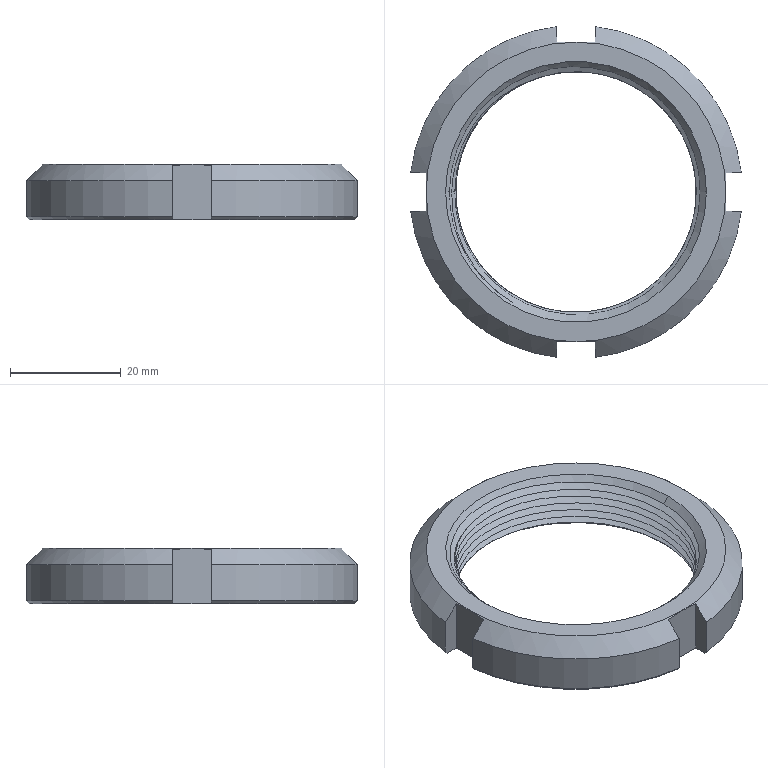Part | SolidWorks | features Chamfer 4, Helix 2, CirPattern 1, Extrusion 1, ICE 1, SweepCut 1 | 1 solid | 32 faces | box 59.59 x 59.59 x 10 mm | volume 10905 mm3 | plane 14 | cone 12 | cylinder 4 | spline 2 | commonest cylinder face diameters 60 x4